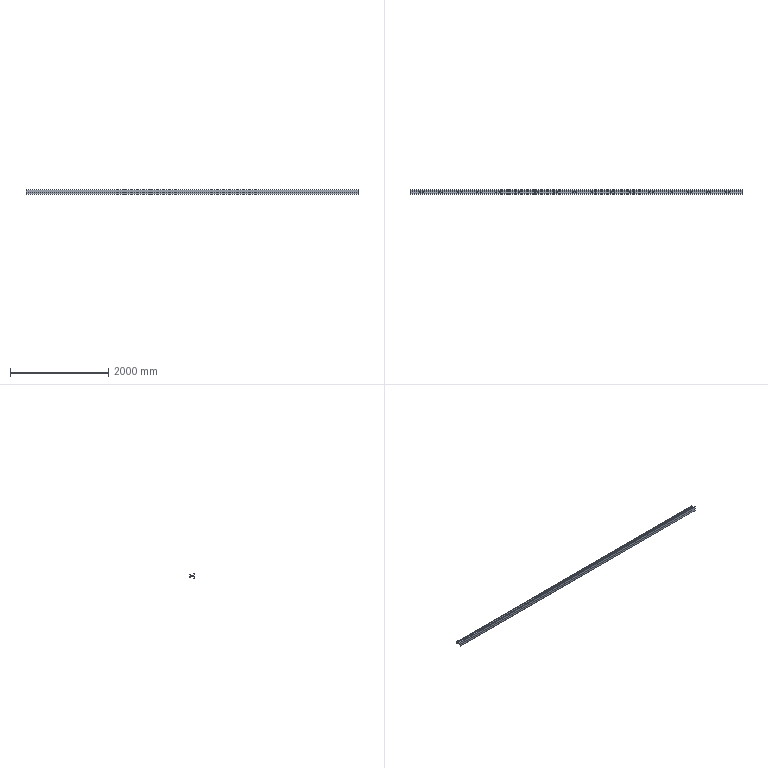Part | SolidWorks | features ICE 1, WeldMemberFeat 1, WeldmentFeature 1 | 1 solid | 94 faces | box 6768 x 93.66 x 93.66 mm | volume 19411583 mm3 | cylinder 78 | plane 16 | commonest cylinder face diameters 17 x68 2 x10